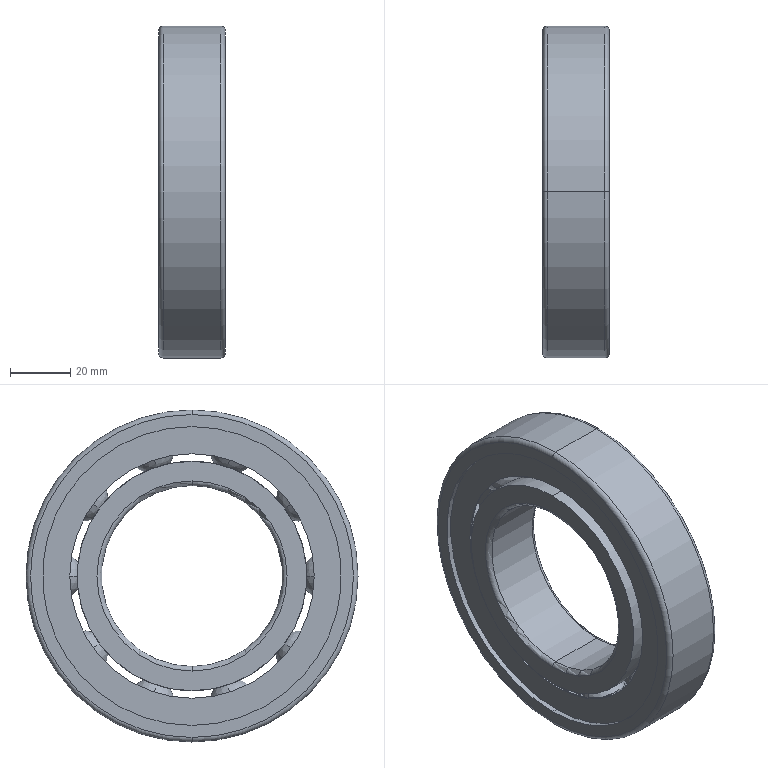Part | STEP file | GB/T276-94 deep groove ball bearing 6212-2Z | 1 solid | 173 faces | box 22 x 110 x 110 mm | volume 94070 mm3 | sphere 80 | torus 41 | plane 28 | cylinder 24 | commonest cylinder face diameters 99 x8 76 x4 80.977 x4 60 x2 83.353 x2 91.647 x2